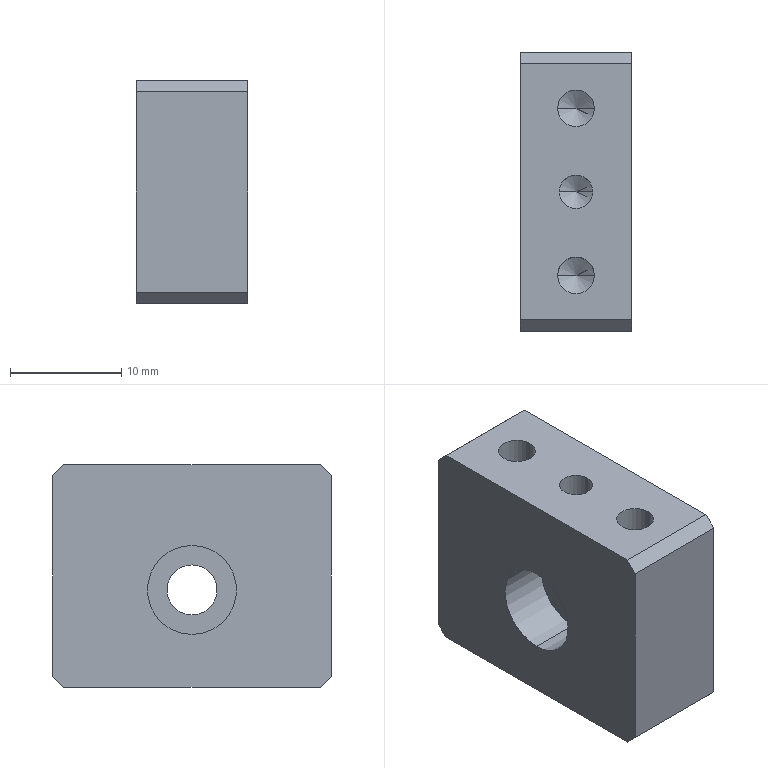Part | SolidWorks | features HoleWzd 3, Chamfer 1, Extrusion 1, ICE 1 | 1 solid | 30 faces | box 10 x 25 x 20 mm | volume 4403 mm3 | cylinder 12 | plane 12 | cone 6 | commonest cylinder face diameters 3.3 x4 3 x2 4.5 x2 8 x2 8.2 x2
STEP:
#1=CARTESIAN_POINT('',(-1.5,12.5,4.));
#2=VERTEX_POINT('',#1);
#3=CARTESIAN_POINT('',(1.5,12.5,4.));
#4=VERTEX_POINT('',#3);
#5=CARTESIAN_POINT('',(0.,12.5,4.));
#6=DIRECTION('',(0.,0.,1.));
#7=DIRECTION('',(1.,0.,0.));
#8=AXIS2_PLACEMENT_3D('',#5,#6,#7);
#9=CIRCLE('',#8,1.5);
#10=EDGE_CURVE('',#2,#4,#9,.T.);
#11=ORIENTED_EDGE('',*,*,#10,.F.);
#12=CARTESIAN_POINT('',(-1.5,12.5,10.));
#13=VERTEX_POINT('',#12);
#14=CARTESIAN_POINT('',(-1.5,12.5,10.));
#15=DIRECTION('',(0.,0.,1.));
#16=VECTOR('',#15,1000.);
#17=LINE('',#14,#16);
#18=EDGE_CURVE('',#2,#13,#17,.T.);
#19=ORIENTED_EDGE('',*,*,#18,.T.);
#20=CARTESIAN_POINT('',(1.5,12.5,10.));
#21=VERTEX_POINT('',#20);
#22=CARTESIAN_POINT('',(0.,12.5,10.));
#23=DIRECTION('',(0.,0.,1.));
#24=DIRECTION('',(1.,0.,0.));
#25=AXIS2_PLACEMENT_3D('',#22,#23,#24);
#26=CIRCLE('',#25,1.5);
#27=EDGE_CURVE('',#13,#21,#26,.T.);
#28=ORIENTED_EDGE('',*,*,#27,.T.);
#29=CARTESIAN_POINT('',(1.5,12.5,10.));
#30=DIRECTION('',(0.,0.,1.));
#31=VECTOR('',#30,1000.);
#32=LINE('',#29,#31);
#33=EDGE_CURVE('',#4,#21,#32,.T.);
#34=ORIENTED_EDGE('',*,*,#33,.F.);
#35=EDGE_LOOP('',(#11,#19,#28,#34));
#36=FACE_OUTER_BOUND('',#35,.T.);
#37=CARTESIAN_POINT('',(0.,12.5,10.));
#38=DIRECTION('',(0.,0.,1.));
#39=DIRECTION('',(1.,0.,0.));
#40=AXIS2_PLACEMENT_3D('',#37,#38,#39);
#41=CYLINDRICAL_SURFACE('',#40,1.5);
#42=ADVANCED_FACE('',(#36),#41,.F.);
#43=CARTESIAN_POINT('',(0.,12.5,3.099));
#44=VERTEX_POINT('',#43);
#45=CARTESIAN_POINT('',(1.5,12.5,4.));
#46=DIRECTION('',(0.8572,0.,0.515));
#47=VECTOR('',#46,1000.);
#48=LINE('',#45,#47);
#49=EDGE_CURVE('',#44,#4,#48,.T.);
#50=ORIENTED_EDGE('',*,*,#49,.F.);
#51=CARTESIAN_POINT('',(-1.5,12.5,4.));
#52=DIRECTION('',(-0.8572,0.,0.515));
#53=VECTOR('',#52,1000.);
#54=LINE('',#51,#53);
#55=EDGE_CURVE('',#44,#2,#54,.T.);
#56=ORIENTED_EDGE('',*,*,#55,.T.);
#57=ORIENTED_EDGE('',*,*,#10,.T.);
#58=EDGE_LOOP('',(#50,#56,#57));
#59=FACE_OUTER_BOUND('',#58,.T.);
#60=CARTESIAN_POINT('',(0.,12.5,4.));
#61=DIRECTION('',(0.,0.,1.));
#62=DIRECTION('',(1.,0.,0.));
#63=AXIS2_PLACEMENT_3D('',#60,#61,#62);
#64=CONICAL_SURFACE('',#63,1.5,1.03);
#65=ADVANCED_FACE('',(#59),#64,.F.);
#66=CARTESIAN_POINT('',(-1.65,20.,-0.1));
#67=VERTEX_POINT('',#66);
#68=CARTESIAN_POINT('',(1.65,20.,-0.1));
#69=VERTEX_POINT('',#68);
#70=CARTESIAN_POINT('',(0.,20.,-0.1));
#71=DIRECTION('',(0.,0.,1.));
#72=DIRECTION('',(1.,0.,0.));
#73=AXIS2_PLACEMENT_3D('',#70,#71,#72);
#74=CIRCLE('',#73,1.65);
#75=EDGE_CURVE('',#67,#69,#74,.T.);
#76=ORIENTED_EDGE('',*,*,#75,.F.);
#77=CARTESIAN_POINT('',(-1.65,20.,10.));
#78=VERTEX_POINT('',#77);
#79=CARTESIAN_POINT('',(-1.65,20.,10.));
#80=DIRECTION('',(0.,0.,1.));
#81=VECTOR('',#80,1000.);
#82=LINE('',#79,#81);
#83=EDGE_CURVE('',#67,#78,#82,.T.);
#84=ORIENTED_EDGE('',*,*,#83,.T.);
#85=CARTESIAN_POINT('',(1.65,20.,10.));
#86=VERTEX_POINT('',#85);
#87=CARTESIAN_POINT('',(0.,20.,10.));
#88=DIRECTION('',(0.,0.,1.));
#89=DIRECTION('',(1.,0.,0.));
#90=AXIS2_PLACEMENT_3D('',#87,#88,#89);
#91=CIRCLE('',#90,1.65);
#92=EDGE_CURVE('',#78,#86,#91,.T.);
#93=ORIENTED_EDGE('',*,*,#92,.T.);
#94=CARTESIAN_POINT('',(1.65,20.,10.));
#95=DIRECTION('',(0.,0.,1.));
#96=VECTOR('',#95,1000.);
#97=LINE('',#94,#96);
#98=EDGE_CURVE('',#69,#86,#97,.T.);
#99=ORIENTED_EDGE('',*,*,#98,.F.);
#100=EDGE_LOOP('',(#76,#84,#93,#99));
#101=FACE_OUTER_BOUND('',#100,.T.);
#102=CARTESIAN_POINT('',(0.,20.,10.));
#103=DIRECTION('',(0.,0.,1.));
#104=DIRECTION('',(1.,0.,0.));
#105=AXIS2_PLACEMENT_3D('',#102,#103,#104);
#106=CYLINDRICAL_SURFACE('',#105,1.65);
#107=ADVANCED_FACE('',(#101),#106,.F.);
#108=CARTESIAN_POINT('',(0.,20.,-1.091));
#109=VERTEX_POINT('',#108);
#110=CARTESIAN_POINT('',(1.65,20.,-0.1));
#111=DIRECTION('',(0.8572,0.,0.515));
#112=VECTOR('',#111,1000.);
#113=LINE('',#110,#112);
#114=EDGE_CURVE('',#109,#69,#113,.T.);
#115=ORIENTED_EDGE('',*,*,#114,.F.);
#116=CARTESIAN_POINT('',(-1.65,20.,-0.1));
#117=DIRECTION('',(-0.8572,0.,0.515));
#118=VECTOR('',#117,1000.);
#119=LINE('',#116,#118);
#120=EDGE_CURVE('',#109,#67,#119,.T.);
#121=ORIENTED_EDGE('',*,*,#120,.T.);
#122=ORIENTED_EDGE('',*,*,#75,.T.);
#123=EDGE_LOOP('',(#115,#121,#122));
#124=FACE_OUTER_BOUND('',#123,.T.);
#125=CARTESIAN_POINT('',(0.,20.,-0.1));
#126=DIRECTION('',(0.,0.,1.));
#127=DIRECTION('',(1.,0.,0.));
#128=AXIS2_PLACEMENT_3D('',#125,#126,#127);
#129=CONICAL_SURFACE('',#128,1.65,1.03);
#130=ADVANCED_FACE('',(#124),#129,.F.);
#131=CARTESIAN_POINT('',(-1.65,5.,-0.1));
#132=VERTEX_POINT('',#131);
#133=CARTESIAN_POINT('',(1.65,5.,-0.1));
#134=VERTEX_POINT('',#133);
#135=CARTESIAN_POINT('',(0.,5.,-0.1));
#136=DIRECTION('',(0.,0.,1.));
#137=DIRECTION('',(1.,0.,0.));
#138=AXIS2_PLACEMENT_3D('',#135,#136,#137);
#139=CIRCLE('',#138,1.65);
#140=EDGE_CURVE('',#132,#134,#139,.T.);
#141=ORIENTED_EDGE('',*,*,#140,.F.);
#142=CARTESIAN_POINT('',(-1.65,5.,10.));
#143=VERTEX_POINT('',#142);
#144=CARTESIAN_POINT('',(-1.65,5.,10.));
#145=DIRECTION('',(0.,0.,1.));
#146=VECTOR('',#145,1000.);
#147=LINE('',#144,#146);
#148=EDGE_CURVE('',#132,#143,#147,.T.);
#149=ORIENTED_EDGE('',*,*,#148,.T.);
#150=CARTESIAN_POINT('',(1.65,5.,10.));
#151=VERTEX_POINT('',#150);
#152=CARTESIAN_POINT('',(0.,5.,10.));
#153=DIRECTION('',(0.,0.,1.));
#154=DIRECTION('',(1.,0.,0.));
#155=AXIS2_PLACEMENT_3D('',#152,#153,#154);
#156=CIRCLE('',#155,1.65);
#157=EDGE_CURVE('',#143,#151,#156,.T.);
#158=ORIENTED_EDGE('',*,*,#157,.T.);
#159=CARTESIAN_POINT('',(1.65,5.,10.));
#160=DIRECTION('',(0.,0.,1.));
#161=VECTOR('',#160,1000.);
#162=LINE('',#159,#161);
#163=EDGE_CURVE('',#134,#151,#162,.T.);
#164=ORIENTED_EDGE('',*,*,#163,.F.);
#165=EDGE_LOOP('',(#141,#149,#158,#164));
#166=FACE_OUTER_BOUND('',#165,.T.);
#167=CARTESIAN_POINT('',(0.,5.,10.));
#168=DIRECTION('',(0.,0.,1.));
#169=DIRECTION('',(1.,0.,0.));
#170=AXIS2_PLACEMENT_3D('',#167,#168,#169);
#171=CYLINDRICAL_SURFACE('',#170,1.65);
#172=ADVANCED_FACE('',(#166),#171,.F.);
#173=CARTESIAN_POINT('',(0.,5.,-1.091));
#174=VERTEX_POINT('',#173);
#175=CARTESIAN_POINT('',(1.65,5.,-0.1));
#176=DIRECTION('',(0.8572,0.,0.515));
#177=VECTOR('',#176,1000.);
#178=LINE('',#175,#177);
#179=EDGE_CURVE('',#174,#134,#178,.T.);
#180=ORIENTED_EDGE('',*,*,#179,.F.);
#181=CARTESIAN_POINT('',(-1.65,5.,-0.1));
#182=DIRECTION('',(-0.8572,0.,0.515));
#183=VECTOR('',#182,1000.);
#184=LINE('',#181,#183);
#185=EDGE_CURVE('',#174,#132,#184,.T.);
#186=ORIENTED_EDGE('',*,*,#185,.T.);
#187=ORIENTED_EDGE('',*,*,#140,.T.);
#188=EDGE_LOOP('',(#180,#186,#187));
#189=FACE_OUTER_BOUND('',#188,.T.);
#190=CARTESIAN_POINT('',(0.,5.,-0.1));
#191=DIRECTION('',(0.,0.,1.));
#192=DIRECTION('',(1.,0.,0.));
#193=AXIS2_PLACEMENT_3D('',#190,#191,#192);
#194=CONICAL_SURFACE('',#193,1.65,1.03);
#195=ADVANCED_FACE('',(#189),#194,.F.);
#196=CARTESIAN_POINT('',(4.,12.5,2.85));
#197=VERTEX_POINT('',#196);
#198=CARTESIAN_POINT('',(4.,12.5,-5.35));
#199=VERTEX_POINT('',#198);
#200=CARTESIAN_POINT('',(4.,12.5,-1.25));
#201=DIRECTION('',(1.,0.,0.));
#202=DIRECTION('',(0.,0.,-1.));
#203=AXIS2_PLACEMENT_3D('',#200,#201,#202);
#204=CIRCLE('',#203,4.1);
#205=EDGE_CURVE('',#197,#199,#204,.T.);
#206=ORIENTED_EDGE('',*,*,#205,.F.);
#207=CARTESIAN_POINT('',(5.,12.5,2.85));
#208=VERTEX_POINT('',#207);
#209=CARTESIAN_POINT('',(4.,12.5,2.85));
#210=DIRECTION('',(1.,0.,0.));
#211=VECTOR('',#210,1000.);
#212=LINE('',#209,#211);
#213=EDGE_CURVE('',#197,#208,#212,.T.);
#214=ORIENTED_EDGE('',*,*,#213,.T.);
#215=CARTESIAN_POINT('',(5.,12.5,-5.35));
#216=VERTEX_POINT('',#215);
#217=CARTESIAN_POINT('',(5.,12.5,-1.25));
#218=DIRECTION('',(1.,0.,0.));
#219=DIRECTION('',(0.,0.,-1.));
#220=AXIS2_PLACEMENT_3D('',#217,#218,#219);
#221=CIRCLE('',#220,4.1);
#222=EDGE_CURVE('',#208,#216,#221,.T.);
#223=ORIENTED_EDGE('',*,*,#222,.T.);
#224=CARTESIAN_POINT('',(4.,12.5,-5.35));
#225=DIRECTION('',(1.,0.,0.));
#226=VECTOR('',#225,1000.);
#227=LINE('',#224,#226);
#228=EDGE_CURVE('',#199,#216,#227,.T.);
#229=ORIENTED_EDGE('',*,*,#228,.F.);
#230=EDGE_LOOP('',(#206,#214,#223,#229));
#231=FACE_OUTER_BOUND('',#230,.T.);
#232=CARTESIAN_POINT('',(4.,12.5,-1.25));
#233=DIRECTION('',(1.,0.,0.));
#234=DIRECTION('',(0.,0.,-1.));
#235=AXIS2_PLACEMENT_3D('',#232,#233,#234);
#236=CYLINDRICAL_SURFACE('',#235,4.1);
#237=ADVANCED_FACE('',(#231),#236,.F.);
#238=CARTESIAN_POINT('',(-0.4,12.5,-5.25));
#239=VERTEX_POINT('',#238);
#240=CARTESIAN_POINT('',(-0.4,12.5,2.75));
#241=VERTEX_POINT('',#240);
#242=CARTESIAN_POINT('',(-0.4,12.5,-1.25));
#243=DIRECTION('',(-1.,0.,0.));
#244=DIRECTION('',(0.,0.,1.));
#245=AXIS2_PLACEMENT_3D('',#242,#243,#244);
#246=CIRCLE('',#245,4.);
#247=EDGE_CURVE('',#239,#241,#246,.T.);
#248=ORIENTED_EDGE('',*,*,#247,.F.);
#249=CARTESIAN_POINT('',(-5.,12.5,-5.25));
#250=VERTEX_POINT('',#249);
#251=CARTESIAN_POINT('',(-5.,12.5,-5.25));
#252=DIRECTION('',(-1.,0.,0.));
#253=VECTOR('',#252,1000.);
#254=LINE('',#251,#253);
#255=EDGE_CURVE('',#239,#250,#254,.T.);
#256=ORIENTED_EDGE('',*,*,#255,.T.);
#257=CARTESIAN_POINT('',(-5.,12.5,2.75));
#258=VERTEX_POINT('',#257);
#259=CARTESIAN_POINT('',(-5.,12.5,-1.25));
#260=DIRECTION('',(-1.,0.,0.));
#261=DIRECTION('',(0.,0.,1.));
#262=AXIS2_PLACEMENT_3D('',#259,#260,#261);
#263=CIRCLE('',#262,4.);
#264=EDGE_CURVE('',#250,#258,#263,.T.);
#265=ORIENTED_EDGE('',*,*,#264,.T.);
#266=CARTESIAN_POINT('',(-5.,12.5,2.75));
#267=DIRECTION('',(-1.,0.,0.));
#268=VECTOR('',#267,1000.);
#269=LINE('',#266,#268);
#270=EDGE_CURVE('',#241,#258,#269,.T.);
#271=ORIENTED_EDGE('',*,*,#270,.F.);
#272=EDGE_LOOP('',(#248,#256,#265,#271));
#273=FACE_OUTER_BOUND('',#272,.T.);
#274=CARTESIAN_POINT('',(-5.,12.5,-1.25));
#275=DIRECTION('',(-1.,0.,0.));
#276=DIRECTION('',(0.,0.,1.));
#277=AXIS2_PLACEMENT_3D('',#274,#275,#276);
#278=CYLINDRICAL_SURFACE('',#277,4.);
#279=ADVANCED_FACE('',(#273),#278,.F.);
#280=CARTESIAN_POINT('',(4.,12.5,-3.5));
#281=VERTEX_POINT('',#280);
#282=CARTESIAN_POINT('',(4.,12.5,1.));
#283=VERTEX_POINT('',#282);
#284=CARTESIAN_POINT('',(4.,12.5,-1.25));
#285=DIRECTION('',(-1.,0.,0.));
#286=DIRECTION('',(0.,0.,-1.));
#287=AXIS2_PLACEMENT_3D('',#284,#285,#286);
#288=CIRCLE('',#287,2.25);
#289=EDGE_CURVE('',#281,#283,#288,.T.);
#290=ORIENTED_EDGE('',*,*,#289,.F.);
#291=CARTESIAN_POINT('',(-0.4,12.5,-3.5));
#292=VERTEX_POINT('',#291);
#293=CARTESIAN_POINT('',(-5.,12.5,-3.5));
#294=DIRECTION('',(-1.,0.,0.));
#295=VECTOR('',#294,1000.);
#296=LINE('',#293,#295);
#297=EDGE_CURVE('',#281,#292,#296,.T.);
#298=ORIENTED_EDGE('',*,*,#297,.T.);
#299=CARTESIAN_POINT('',(-0.4,12.5,1.));
#300=VERTEX_POINT('',#299);
#301=CARTESIAN_POINT('',(-0.4,12.5,-1.25));
#302=DIRECTION('',(-1.,0.,0.));
#303=DIRECTION('',(0.,0.,1.));
#304=AXIS2_PLACEMENT_3D('',#301,#302,#303);
#305=CIRCLE('',#304,2.25);
#306=EDGE_CURVE('',#292,#300,#305,.T.);
#307=ORIENTED_EDGE('',*,*,#306,.T.);
#308=CARTESIAN_POINT('',(-5.,12.5,1.));
#309=DIRECTION('',(-1.,0.,0.));
#310=VECTOR('',#309,1000.);
#311=LINE('',#308,#310);
#312=EDGE_CURVE('',#283,#300,#311,.T.);
#313=ORIENTED_EDGE('',*,*,#312,.F.);
#314=EDGE_LOOP('',(#290,#298,#307,#313));
#315=FACE_OUTER_BOUND('',#314,.T.);
#316=CARTESIAN_POINT('',(-5.,12.5,-1.25));
#317=DIRECTION('',(-1.,0.,0.));
#318=DIRECTION('',(0.,0.,1.));
#319=AXIS2_PLACEMENT_3D('',#316,#317,#318);
#320=CYLINDRICAL_SURFACE('',#319,2.25);
#321=ADVANCED_FACE('',(#315),#320,.F.);
#322=ORIENTED_EDGE('',*,*,#297,.F.);
#323=CARTESIAN_POINT('',(4.,12.5,-1.25));
#324=DIRECTION('',(-1.,0.,0.));
#325=DIRECTION('',(0.,0.,-1.));
#326=AXIS2_PLACEMENT_3D('',#323,#324,#325);
#327=CIRCLE('',#326,2.25);
#328=EDGE_CURVE('',#283,#281,#327,.T.);
#329=ORIENTED_EDGE('',*,*,#328,.F.);
#330=ORIENTED_EDGE('',*,*,#312,.T.);
#331=CARTESIAN_POINT('',(-0.4,12.5,-1.25));
#332=DIRECTION('',(-1.,0.,0.));
#333=DIRECTION('',(0.,0.,1.));
#334=AXIS2_PLACEMENT_3D('',#331,#332,#333);
#335=CIRCLE('',#334,2.25);
#336=EDGE_CURVE('',#300,#292,#335,.T.);
#337=ORIENTED_EDGE('',*,*,#336,.T.);
#338=EDGE_LOOP('',(#322,#329,#330,#337));
#339=FACE_OUTER_BOUND('',#338,.T.);
#340=CARTESIAN_POINT('',(-5.,12.5,-1.25));
#341=DIRECTION('',(-1.,0.,0.));
#342=DIRECTION('',(0.,0.,1.));
#343=AXIS2_PLACEMENT_3D('',#340,#341,#342);
#344=CYLINDRICAL_SURFACE('',#343,2.25);
#345=ADVANCED_FACE('',(#339),#344,.F.);
#346=CARTESIAN_POINT('',(5.,12.5,-1.25));
#347=DIRECTION('',(1.,0.,0.));
#348=DIRECTION('',(0.,0.,-1.));
#349=AXIS2_PLACEMENT_3D('',#346,#347,#348);
#350=CIRCLE('',#349,4.1);
#351=EDGE_CURVE('',#216,#208,#350,.T.);
#352=ORIENTED_EDGE('',*,*,#351,.F.);
#353=ORIENTED_EDGE('',*,*,#222,.F.);
#354=EDGE_LOOP('',(#352,#353));
#355=FACE_BOUND('',#354,.T.);
#356=CARTESIAN_POINT('',(5.,24.,10.));
#357=VERTEX_POINT('',#356);
#358=CARTESIAN_POINT('',(5.,1.,10.));
#359=VERTEX_POINT('',#358);
#360=CARTESIAN_POINT('',(5.,25.,10.));
#361=DIRECTION('',(0.,-1.,0.));
#362=VECTOR('',#361,1000.);
#363=LINE('',#360,#362);
#364=EDGE_CURVE('',#357,#359,#363,.T.);
#365=ORIENTED_EDGE('',*,*,#364,.T.);
#366=CARTESIAN_POINT('',(5.,0.,9.));
#367=VERTEX_POINT('',#366);
#368=CARTESIAN_POINT('',(5.,1.,10.));
#369=DIRECTION('',(0.,-0.7071,-0.7071));
#370=VECTOR('',#369,1000.);
#371=LINE('',#368,#370);
#372=EDGE_CURVE('',#359,#367,#371,.T.);
#373=ORIENTED_EDGE('',*,*,#372,.T.);
#374=CARTESIAN_POINT('',(5.,0.,-9.));
#375=VERTEX_POINT('',#374);
#376=CARTESIAN_POINT('',(5.,0.,-10.));
#377=DIRECTION('',(0.,0.,-1.));
#378=VECTOR('',#377,1000.);
#379=LINE('',#376,#378);
#380=EDGE_CURVE('',#367,#375,#379,.T.);
#381=ORIENTED_EDGE('',*,*,#380,.T.);
#382=CARTESIAN_POINT('',(5.,1.,-10.));
#383=VERTEX_POINT('',#382);
#384=CARTESIAN_POINT('',(5.,1.,-10.));
#385=DIRECTION('',(0.,0.7071,-0.7071));
#386=VECTOR('',#385,1000.);
#387=LINE('',#384,#386);
#388=EDGE_CURVE('',#375,#383,#387,.T.);
#389=ORIENTED_EDGE('',*,*,#388,.T.);
#390=CARTESIAN_POINT('',(5.,24.,-10.));
#391=VERTEX_POINT('',#390);
#392=CARTESIAN_POINT('',(5.,25.,-10.));
#393=DIRECTION('',(0.,-1.,0.));
#394=VECTOR('',#393,1000.);
#395=LINE('',#392,#394);
#396=EDGE_CURVE('',#391,#383,#395,.T.);
#397=ORIENTED_EDGE('',*,*,#396,.F.);
#398=CARTESIAN_POINT('',(5.,25.,-9.));
#399=VERTEX_POINT('',#398);
#400=CARTESIAN_POINT('',(5.,25.,-9.));
#401=DIRECTION('',(0.,0.7071,0.7071));
#402=VECTOR('',#401,1000.);
#403=LINE('',#400,#402);
#404=EDGE_CURVE('',#391,#399,#403,.T.);
#405=ORIENTED_EDGE('',*,*,#404,.T.);
#406=CARTESIAN_POINT('',(5.,25.,9.));
#407=VERTEX_POINT('',#406);
#408=CARTESIAN_POINT('',(5.,25.,-10.));
#409=DIRECTION('',(0.,0.,-1.));
#410=VECTOR('',#409,1000.);
#411=LINE('',#408,#410);
#412=EDGE_CURVE('',#407,#399,#411,.T.);
#413=ORIENTED_EDGE('',*,*,#412,.F.);
#414=CARTESIAN_POINT('',(5.,25.,9.));
#415=DIRECTION('',(0.,-0.7071,0.7071));
#416=VECTOR('',#415,1000.);
#417=LINE('',#414,#416);
#418=EDGE_CURVE('',#407,#357,#417,.T.);
#419=ORIENTED_EDGE('',*,*,#418,.T.);
#420=EDGE_LOOP('',(#365,#373,#381,#389,#397,#405,#413,#419));
#421=FACE_OUTER_BOUND('',#420,.T.);
#422=CARTESIAN_POINT('',(5.,25.,-10.));
#423=DIRECTION('',(-1.,0.,0.));
#424=DIRECTION('',(0.,0.,1.));
#425=AXIS2_PLACEMENT_3D('',#422,#423,#424);
#426=PLANE('',#425);
#427=ADVANCED_FACE('',(#355,#421),#426,.F.);
#428=ORIENTED_EDGE('',*,*,#396,.T.);
#429=CARTESIAN_POINT('',(-5.,1.,-10.));
#430=VERTEX_POINT('',#429);
#431=CARTESIAN_POINT('',(-5.,1.,-10.));
#432=DIRECTION('',(-1.,0.,0.));
#433=VECTOR('',#432,1000.);
#434=LINE('',#431,#433);
#435=EDGE_CURVE('',#383,#430,#434,.T.);
#436=ORIENTED_EDGE('',*,*,#435,.T.);
#437=CARTESIAN_POINT('',(-5.,24.,-10.));
#438=VERTEX_POINT('',#437);
#439=CARTESIAN_POINT('',(-5.,25.,-10.));
#440=DIRECTION('',(0.,-1.,0.));
#441=VECTOR('',#440,1000.);
#442=LINE('',#439,#441);
#443=EDGE_CURVE('',#438,#430,#442,.T.);
#444=ORIENTED_EDGE('',*,*,#443,.F.);
#445=CARTESIAN_POINT('',(5.,24.,-10.));
#446=DIRECTION('',(1.,0.,0.));
#447=VECTOR('',#446,1000.);
#448=LINE('',#445,#447);
#449=EDGE_CURVE('',#438,#391,#448,.T.);
#450=ORIENTED_EDGE('',*,*,#449,.T.);
#451=EDGE_LOOP('',(#428,#436,#444,#450));
#452=FACE_OUTER_BOUND('',#451,.T.);
#453=CARTESIAN_POINT('',(-5.,25.,-10.));
#454=DIRECTION('',(0.,0.,1.));
#455=DIRECTION('',(1.,0.,0.));
#456=AXIS2_PLACEMENT_3D('',#453,#454,#455);
#457=PLANE('',#456);
#458=ADVANCED_FACE('',(#452),#457,.F.);
#459=CARTESIAN_POINT('',(-5.,12.5,-1.25));
#460=DIRECTION('',(-1.,0.,0.));
#461=DIRECTION('',(0.,0.,1.));
#462=AXIS2_PLACEMENT_3D('',#459,#460,#461);
#463=CIRCLE('',#462,4.);
#464=EDGE_CURVE('',#258,#250,#463,.T.);
#465=ORIENTED_EDGE('',*,*,#464,.F.);
#466=ORIENTED_EDGE('',*,*,#264,.F.);
#467=EDGE_LOOP('',(#465,#466));
#468=FACE_BOUND('',#467,.T.);
#469=CARTESIAN_POINT('',(-5.,0.,-9.));
#470=VERTEX_POINT('',#469);
#471=CARTESIAN_POINT('',(-5.,0.,9.));
#472=VERTEX_POINT('',#471);
#473=CARTESIAN_POINT('',(-5.,0.,-10.));
#474=DIRECTION('',(0.,0.,1.));
#475=VECTOR('',#474,1000.);
#476=LINE('',#473,#475);
#477=EDGE_CURVE('',#470,#472,#476,.T.);
#478=ORIENTED_EDGE('',*,*,#477,.T.);
#479=CARTESIAN_POINT('',(-5.,1.,10.));
#480=VERTEX_POINT('',#479);
#481=CARTESIAN_POINT('',(-5.,1.,10.));
#482=DIRECTION('',(0.,0.7071,0.7071));
#483=VECTOR('',#482,1000.);
#484=LINE('',#481,#483);
#485=EDGE_CURVE('',#472,#480,#484,.T.);
#486=ORIENTED_EDGE('',*,*,#485,.T.);
#487=CARTESIAN_POINT('',(-5.,24.,10.));
#488=VERTEX_POINT('',#487);
#489=CARTESIAN_POINT('',(-5.,25.,10.));
#490=DIRECTION('',(0.,-1.,0.));
#491=VECTOR('',#490,1000.);
#492=LINE('',#489,#491);
#493=EDGE_CURVE('',#488,#480,#492,.T.);
#494=ORIENTED_EDGE('',*,*,#493,.F.);
#495=CARTESIAN_POINT('',(-5.,25.,9.));
#496=VERTEX_POINT('',#495);
#497=CARTESIAN_POINT('',(-5.,25.,9.));
#498=DIRECTION('',(0.,0.7071,-0.7071));
#499=VECTOR('',#498,1000.);
#500=LINE('',#497,#499);
#501=EDGE_CURVE('',#488,#496,#500,.T.);
#502=ORIENTED_EDGE('',*,*,#501,.T.);
#503=CARTESIAN_POINT('',(-5.,25.,-9.));
#504=VERTEX_POINT('',#503);
#505=CARTESIAN_POINT('',(-5.,25.,-10.));
#506=DIRECTION('',(0.,0.,1.));
#507=VECTOR('',#506,1000.);
#508=LINE('',#505,#507);
#509=EDGE_CURVE('',#504,#496,#508,.T.);
#510=ORIENTED_EDGE('',*,*,#509,.F.);
#511=CARTESIAN_POINT('',(-5.,25.,-9.));
#512=DIRECTION('',(0.,-0.7071,-0.7071));
#513=VECTOR('',#512,1000.);
#514=LINE('',#511,#513);
#515=EDGE_CURVE('',#504,#438,#514,.T.);
#516=ORIENTED_EDGE('',*,*,#515,.T.);
#517=ORIENTED_EDGE('',*,*,#443,.T.);
#518=CARTESIAN_POINT('',(-5.,1.,-10.));
#519=DIRECTION('',(0.,-0.7071,0.7071));
#520=VECTOR('',#519,1000.);
#521=LINE('',#518,#520);
#522=EDGE_CURVE('',#430,#470,#521,.T.);
#523=ORIENTED_EDGE('',*,*,#522,.T.);
#524=EDGE_LOOP('',(#478,#486,#494,#502,#510,#516,#517,#523));
#525=FACE_OUTER_BOUND('',#524,.T.);
#526=CARTESIAN_POINT('',(-5.,25.,-10.));
#527=DIRECTION('',(1.,0.,0.));
#528=DIRECTION('',(0.,0.,-1.));
#529=AXIS2_PLACEMENT_3D('',#526,#527,#528);
#530=PLANE('',#529);
#531=ADVANCED_FACE('',(#468,#525),#530,.F.);
#532=CARTESIAN_POINT('',(0.,12.5,10.));
#533=DIRECTION('',(0.,0.,1.));
#534=DIRECTION('',(1.,0.,0.));
#535=AXIS2_PLACEMENT_3D('',#532,#533,#534);
#536=CIRCLE('',#535,1.5);
#537=EDGE_CURVE('',#21,#13,#536,.T.);
#538=ORIENTED_EDGE('',*,*,#537,.F.);
#539=ORIENTED_EDGE('',*,*,#27,.F.);
#540=EDGE_LOOP('',(#538,#539));
#541=FACE_BOUND('',#540,.T.);
#542=CARTESIAN_POINT('',(0.,20.,10.));
#543=DIRECTION('',(0.,0.,1.));
#544=DIRECTION('',(1.,0.,0.));
#545=AXIS2_PLACEMENT_3D('',#542,#543,#544);
#546=CIRCLE('',#545,1.65);
#547=EDGE_CURVE('',#86,#78,#546,.T.);
#548=ORIENTED_EDGE('',*,*,#547,.F.);
#549=ORIENTED_EDGE('',*,*,#92,.F.);
#550=EDGE_LOOP('',(#548,#549));
#551=FACE_BOUND('',#550,.T.);
#552=CARTESIAN_POINT('',(0.,5.,10.));
#553=DIRECTION('',(0.,0.,1.));
#554=DIRECTION('',(1.,0.,0.));
#555=AXIS2_PLACEMENT_3D('',#552,#553,#554);
#556=CIRCLE('',#555,1.65);
#557=EDGE_CURVE('',#151,#143,#556,.T.);
#558=ORIENTED_EDGE('',*,*,#557,.F.);
#559=ORIENTED_EDGE('',*,*,#157,.F.);
#560=EDGE_LOOP('',(#558,#559));
#561=FACE_BOUND('',#560,.T.);
#562=ORIENTED_EDGE('',*,*,#493,.T.);
#563=CARTESIAN_POINT('',(-5.,1.,10.));
#564=DIRECTION('',(1.,0.,0.));
#565=VECTOR('',#564,1000.);
#566=LINE('',#563,#565);
#567=EDGE_CURVE('',#480,#359,#566,.T.);
#568=ORIENTED_EDGE('',*,*,#567,.T.);
#569=ORIENTED_EDGE('',*,*,#364,.F.);
#570=CARTESIAN_POINT('',(-5.,24.,10.));
#571=DIRECTION('',(-1.,0.,0.));
#572=VECTOR('',#571,1000.);
#573=LINE('',#570,#572);
#574=EDGE_CURVE('',#357,#488,#573,.T.);
#575=ORIENTED_EDGE('',*,*,#574,.T.);
#576=EDGE_LOOP('',(#562,#568,#569,#575));
#577=FACE_OUTER_BOUND('',#576,.T.);
#578=CARTESIAN_POINT('',(-5.,25.,10.));
#579=DIRECTION('',(0.,0.,-1.));
#580=DIRECTION('',(-1.,0.,0.));
#581=AXIS2_PLACEMENT_3D('',#578,#579,#580);
#582=PLANE('',#581);
#583=ADVANCED_FACE('',(#541,#551,#561,#577),#582,.F.);
#584=ORIENTED_EDGE('',*,*,#412,.T.);
#585=CARTESIAN_POINT('',(-5.,25.,-9.));
#586=DIRECTION('',(-1.,0.,0.));
#587=VECTOR('',#586,1000.);
#588=LINE('',#585,#587);
#589=EDGE_CURVE('',#399,#504,#588,.T.);
#590=ORIENTED_EDGE('',*,*,#589,.T.);
#591=ORIENTED_EDGE('',*,*,#509,.T.);
#592=CARTESIAN_POINT('',(5.,25.,9.));
#593=DIRECTION('',(1.,0.,0.));
#594=VECTOR('',#593,1000.);
#595=LINE('',#592,#594);
#596=EDGE_CURVE('',#496,#407,#595,.T.);
#597=ORIENTED_EDGE('',*,*,#596,.T.);
#598=EDGE_LOOP('',(#584,#590,#591,#597));
#599=FACE_OUTER_BOUND('',#598,.T.);
#600=CARTESIAN_POINT('',(0.,25.,0.));
#601=DIRECTION('',(0.,1.,0.));
#602=DIRECTION('',(0.,0.,1.));
#603=AXIS2_PLACEMENT_3D('',#600,#601,#602);
#604=PLANE('',#603);
#605=ADVANCED_FACE('',(#599),#604,.T.);
#606=ORIENTED_EDGE('',*,*,#380,.F.);
#607=CARTESIAN_POINT('',(0.,0.,9.));
#608=DIRECTION('',(-1.,0.,0.));
#609=VECTOR('',#608,1000.);
#610=LINE('',#607,#609);
#611=EDGE_CURVE('',#367,#472,#610,.T.);
#612=ORIENTED_EDGE('',*,*,#611,.T.);
#613=ORIENTED_EDGE('',*,*,#477,.F.);
#614=CARTESIAN_POINT('',(0.,0.,-9.));
#615=DIRECTION('',(1.,0.,0.));
#616=VECTOR('',#615,1000.);
#617=LINE('',#614,#616);
#618=EDGE_CURVE('',#470,#375,#617,.T.);
#619=ORIENTED_EDGE('',*,*,#618,.T.);
#620=EDGE_LOOP('',(#606,#612,#613,#619));
#621=FACE_OUTER_BOUND('',#620,.T.);
#622=CARTESIAN_POINT('',(0.,0.,0.));
#623=DIRECTION('',(0.,1.,0.));
#624=DIRECTION('',(0.,0.,1.));
#625=AXIS2_PLACEMENT_3D('',#622,#623,#624);
#626=PLANE('',#625);
#627=ADVANCED_FACE('',(#621),#626,.F.);
#628=ORIENTED_EDGE('',*,*,#336,.F.);
#629=ORIENTED_EDGE('',*,*,#306,.F.);
#630=EDGE_LOOP('',(#628,#629));
#631=FACE_BOUND('',#630,.T.);
#632=CARTESIAN_POINT('',(-0.4,12.5,-1.25));
#633=DIRECTION('',(-1.,0.,0.));
#634=DIRECTION('',(0.,0.,1.));
#635=AXIS2_PLACEMENT_3D('',#632,#633,#634);
#636=CIRCLE('',#635,4.);
#637=EDGE_CURVE('',#241,#239,#636,.T.);
#638=ORIENTED_EDGE('',*,*,#637,.T.);
#639=ORIENTED_EDGE('',*,*,#247,.T.);
#640=EDGE_LOOP('',(#638,#639));
#641=FACE_OUTER_BOUND('',#640,.T.);
#642=CARTESIAN_POINT('',(-0.4,14.75,-1.25));
#643=DIRECTION('',(1.,0.,0.));
#644=DIRECTION('',(0.,0.,-1.));
#645=AXIS2_PLACEMENT_3D('',#642,#643,#644);
#646=PLANE('',#645);
#647=ADVANCED_FACE('',(#631,#641),#646,.F.);
#648=ORIENTED_EDGE('',*,*,#255,.F.);
#649=ORIENTED_EDGE('',*,*,#637,.F.);
#650=ORIENTED_EDGE('',*,*,#270,.T.);
#651=ORIENTED_EDGE('',*,*,#464,.T.);
#652=EDGE_LOOP('',(#648,#649,#650,#651));
#653=FACE_OUTER_BOUND('',#652,.T.);
#654=CARTESIAN_POINT('',(-5.,12.5,-1.25));
#655=DIRECTION('',(-1.,0.,0.));
#656=DIRECTION('',(0.,0.,1.));
#657=AXIS2_PLACEMENT_3D('',#654,#655,#656);
#658=CYLINDRICAL_SURFACE('',#657,4.);
#659=ADVANCED_FACE('',(#653),#658,.F.);
#660=CARTESIAN_POINT('',(4.,12.5,-1.25));
#661=DIRECTION('',(1.,0.,0.));
#662=DIRECTION('',(0.,0.,-1.));
#663=AXIS2_PLACEMENT_3D('',#660,#661,#662);
#664=CIRCLE('',#663,4.1);
#665=EDGE_CURVE('',#199,#197,#664,.T.);
#666=ORIENTED_EDGE('',*,*,#665,.T.);
#667=ORIENTED_EDGE('',*,*,#205,.T.);
#668=EDGE_LOOP('',(#666,#667));
#669=FACE_OUTER_BOUND('',#668,.T.);
#670=ORIENTED_EDGE('',*,*,#328,.T.);
#671=ORIENTED_EDGE('',*,*,#289,.T.);
#672=EDGE_LOOP('',(#670,#671));
#673=FACE_BOUND('',#672,.T.);
#674=CARTESIAN_POINT('',(4.,12.5,-1.25));
#675=DIRECTION('',(1.,0.,0.));
#676=DIRECTION('',(0.,0.,-1.));
#677=AXIS2_PLACEMENT_3D('',#674,#675,#676);
#678=PLANE('',#677);
#679=ADVANCED_FACE('',(#669,#673),#678,.T.);
#680=ORIENTED_EDGE('',*,*,#213,.F.);
#681=ORIENTED_EDGE('',*,*,#665,.F.);
#682=ORIENTED_EDGE('',*,*,#228,.T.);
#683=ORIENTED_EDGE('',*,*,#351,.T.);
#684=EDGE_LOOP('',(#680,#681,#682,#683));
#685=FACE_OUTER_BOUND('',#684,.T.);
#686=CARTESIAN_POINT('',(4.,12.5,-1.25));
#687=DIRECTION('',(1.,0.,0.));
#688=DIRECTION('',(0.,0.,-1.));
#689=AXIS2_PLACEMENT_3D('',#686,#687,#688);
#690=CYLINDRICAL_SURFACE('',#689,4.1);
#691=ADVANCED_FACE('',(#685),#690,.F.);
#692=ORIENTED_EDGE('',*,*,#185,.F.);
#693=ORIENTED_EDGE('',*,*,#179,.T.);
#694=CARTESIAN_POINT('',(0.,5.,-0.1));
#695=DIRECTION('',(0.,0.,1.));
#696=DIRECTION('',(1.,0.,0.));
#697=AXIS2_PLACEMENT_3D('',#694,#695,#696);
#698=CIRCLE('',#697,1.65);
#699=EDGE_CURVE('',#134,#132,#698,.T.);
#700=ORIENTED_EDGE('',*,*,#699,.T.);
#701=EDGE_LOOP('',(#692,#693,#700));
#702=FACE_OUTER_BOUND('',#701,.T.);
#703=CARTESIAN_POINT('',(0.,5.,-0.1));
#704=DIRECTION('',(0.,0.,1.));
#705=DIRECTION('',(1.,0.,0.));
#706=AXIS2_PLACEMENT_3D('',#703,#704,#705);
#707=CONICAL_SURFACE('',#706,1.65,1.03);
#708=ADVANCED_FACE('',(#702),#707,.F.);
#709=ORIENTED_EDGE('',*,*,#148,.F.);
#710=ORIENTED_EDGE('',*,*,#699,.F.);
#711=ORIENTED_EDGE('',*,*,#163,.T.);
#712=ORIENTED_EDGE('',*,*,#557,.T.);
#713=EDGE_LOOP('',(#709,#710,#711,#712));
#714=FACE_OUTER_BOUND('',#713,.T.);
#715=CARTESIAN_POINT('',(0.,5.,10.));
#716=DIRECTION('',(0.,0.,1.));
#717=DIRECTION('',(1.,0.,0.));
#718=AXIS2_PLACEMENT_3D('',#715,#716,#717);
#719=CYLINDRICAL_SURFACE('',#718,1.65);
#720=ADVANCED_FACE('',(#714),#719,.F.);
#721=ORIENTED_EDGE('',*,*,#120,.F.);
#722=ORIENTED_EDGE('',*,*,#114,.T.);
#723=CARTESIAN_POINT('',(0.,20.,-0.1));
#724=DIRECTION('',(0.,0.,1.));
#725=DIRECTION('',(1.,0.,0.));
#726=AXIS2_PLACEMENT_3D('',#723,#724,#725);
#727=CIRCLE('',#726,1.65);
#728=EDGE_CURVE('',#69,#67,#727,.T.);
#729=ORIENTED_EDGE('',*,*,#728,.T.);
#730=EDGE_LOOP('',(#721,#722,#729));
#731=FACE_OUTER_BOUND('',#730,.T.);
#732=CARTESIAN_POINT('',(0.,20.,-0.1));
#733=DIRECTION('',(0.,0.,1.));
#734=DIRECTION('',(1.,0.,0.));
#735=AXIS2_PLACEMENT_3D('',#732,#733,#734);
#736=CONICAL_SURFACE('',#735,1.65,1.03);
#737=ADVANCED_FACE('',(#731),#736,.F.);
#738=ORIENTED_EDGE('',*,*,#83,.F.);
#739=ORIENTED_EDGE('',*,*,#728,.F.);
#740=ORIENTED_EDGE('',*,*,#98,.T.);
#741=ORIENTED_EDGE('',*,*,#547,.T.);
#742=EDGE_LOOP('',(#738,#739,#740,#741));
#743=FACE_OUTER_BOUND('',#742,.T.);
#744=CARTESIAN_POINT('',(0.,20.,10.));
#745=DIRECTION('',(0.,0.,1.));
#746=DIRECTION('',(1.,0.,0.));
#747=AXIS2_PLACEMENT_3D('',#744,#745,#746);
#748=CYLINDRICAL_SURFACE('',#747,1.65);
#749=ADVANCED_FACE('',(#743),#748,.F.);
#750=ORIENTED_EDGE('',*,*,#55,.F.);
#751=ORIENTED_EDGE('',*,*,#49,.T.);
#752=CARTESIAN_POINT('',(0.,12.5,4.));
#753=DIRECTION('',(0.,0.,1.));
#754=DIRECTION('',(1.,0.,0.));
#755=AXIS2_PLACEMENT_3D('',#752,#753,#754);
#756=CIRCLE('',#755,1.5);
#757=EDGE_CURVE('',#4,#2,#756,.T.);
#758=ORIENTED_EDGE('',*,*,#757,.T.);
#759=EDGE_LOOP('',(#750,#751,#758));
#760=FACE_OUTER_BOUND('',#759,.T.);
#761=CARTESIAN_POINT('',(0.,12.5,4.));
#762=DIRECTION('',(0.,0.,1.));
#763=DIRECTION('',(1.,0.,0.));
#764=AXIS2_PLACEMENT_3D('',#761,#762,#763);
#765=CONICAL_SURFACE('',#764,1.5,1.03);
#766=ADVANCED_FACE('',(#760),#765,.F.);
#767=ORIENTED_EDGE('',*,*,#18,.F.);
#768=ORIENTED_EDGE('',*,*,#757,.F.);
#769=ORIENTED_EDGE('',*,*,#33,.T.);
#770=ORIENTED_EDGE('',*,*,#537,.T.);
#771=EDGE_LOOP('',(#767,#768,#769,#770));
#772=FACE_OUTER_BOUND('',#771,.T.);
#773=CARTESIAN_POINT('',(0.,12.5,10.));
#774=DIRECTION('',(0.,0.,1.));
#775=DIRECTION('',(1.,0.,0.));
#776=AXIS2_PLACEMENT_3D('',#773,#774,#775);
#777=CYLINDRICAL_SURFACE('',#776,1.5);
#778=ADVANCED_FACE('',(#772),#777,.F.);
#779=ORIENTED_EDGE('',*,*,#485,.F.);
#780=ORIENTED_EDGE('',*,*,#611,.F.);
#781=ORIENTED_EDGE('',*,*,#372,.F.);
#782=ORIENTED_EDGE('',*,*,#567,.F.);
#783=EDGE_LOOP('',(#779,#780,#781,#782));
#784=FACE_OUTER_BOUND('',#783,.T.);
#785=CARTESIAN_POINT('',(-5.,1.,10.));
#786=DIRECTION('',(0.,0.7071,-0.7071));
#787=DIRECTION('',(1.,0.,0.));
#788=AXIS2_PLACEMENT_3D('',#785,#786,#787);
#789=PLANE('',#788);
#790=ADVANCED_FACE('',(#784),#789,.F.);
#791=ORIENTED_EDGE('',*,*,#388,.F.);
#792=ORIENTED_EDGE('',*,*,#618,.F.);
#793=ORIENTED_EDGE('',*,*,#522,.F.);
#794=ORIENTED_EDGE('',*,*,#435,.F.);
#795=EDGE_LOOP('',(#791,#792,#793,#794));
#796=FACE_OUTER_BOUND('',#795,.T.);
#797=CARTESIAN_POINT('',(-5.,1.,-10.));
#798=DIRECTION('',(0.,0.7071,0.7071));
#799=DIRECTION('',(-1.,0.,0.));
#800=AXIS2_PLACEMENT_3D('',#797,#798,#799);
#801=PLANE('',#800);
#802=ADVANCED_FACE('',(#796),#801,.F.);
#803=ORIENTED_EDGE('',*,*,#404,.F.);
#804=ORIENTED_EDGE('',*,*,#449,.F.);
#805=ORIENTED_EDGE('',*,*,#515,.F.);
#806=ORIENTED_EDGE('',*,*,#589,.F.);
#807=EDGE_LOOP('',(#803,#804,#805,#806));
#808=FACE_OUTER_BOUND('',#807,.T.);
#809=CARTESIAN_POINT('',(0.,25.,-9.));
#810=DIRECTION('',(0.,0.7071,-0.7071));
#811=DIRECTION('',(1.,0.,0.));
#812=AXIS2_PLACEMENT_3D('',#809,#810,#811);
#813=PLANE('',#812);
#814=ADVANCED_FACE('',(#808),#813,.T.);
#815=ORIENTED_EDGE('',*,*,#501,.F.);
#816=ORIENTED_EDGE('',*,*,#574,.F.);
#817=ORIENTED_EDGE('',*,*,#418,.F.);
#818=ORIENTED_EDGE('',*,*,#596,.F.);
#819=EDGE_LOOP('',(#815,#816,#817,#818));
#820=FACE_OUTER_BOUND('',#819,.T.);
#821=CARTESIAN_POINT('',(0.,25.,9.));
#822=DIRECTION('',(0.,0.7071,0.7071));
#823=DIRECTION('',(-1.,0.,0.));
#824=AXIS2_PLACEMENT_3D('',#821,#822,#823);
#825=PLANE('',#824);
#826=ADVANCED_FACE('',(#820),#825,.T.);
#827=CLOSED_SHELL('',(#42,#65,#107,#130,#172,#195,#237,#279,#321,#345,#427,#458,#531,#583,#605,#627,#647,#659,#679,#691,#708,#720,#737,#749,#766,#778,#790,#802,#814,#826));
#828=MANIFOLD_SOLID_BREP('',#827);
#829=CARTESIAN_POINT('',(0.,0.,0.));
#830=DIRECTION('',(0.,0.,1.));
#831=DIRECTION('',(1.,0.,0.));
#832=AXIS2_PLACEMENT_3D('',#829,#830,#831);
#833=(LENGTH_UNIT()NAMED_UNIT(*)SI_UNIT(.MILLI.,.METRE.));
#834=UNCERTAINTY_MEASURE_WITH_UNIT(LENGTH_MEASURE(0.00001),#833,'','');
#835=(NAMED_UNIT(*)PLANE_ANGLE_UNIT()SI_UNIT($,.RADIAN.));
#836=(NAMED_UNIT(*)SI_UNIT($,.STERADIAN.)SOLID_ANGLE_UNIT());
#837=(GEOMETRIC_REPRESENTATION_CONTEXT(3)GLOBAL_UNCERTAINTY_ASSIGNED_CONTEXT((#834))GLOBAL_UNIT_ASSIGNED_CONTEXT((#833,#835,#836))REPRESENTATION_CONTEXT('',''));
#838=ADVANCED_BREP_SHAPE_REPRESENTATION('',(#828,#832),#837);